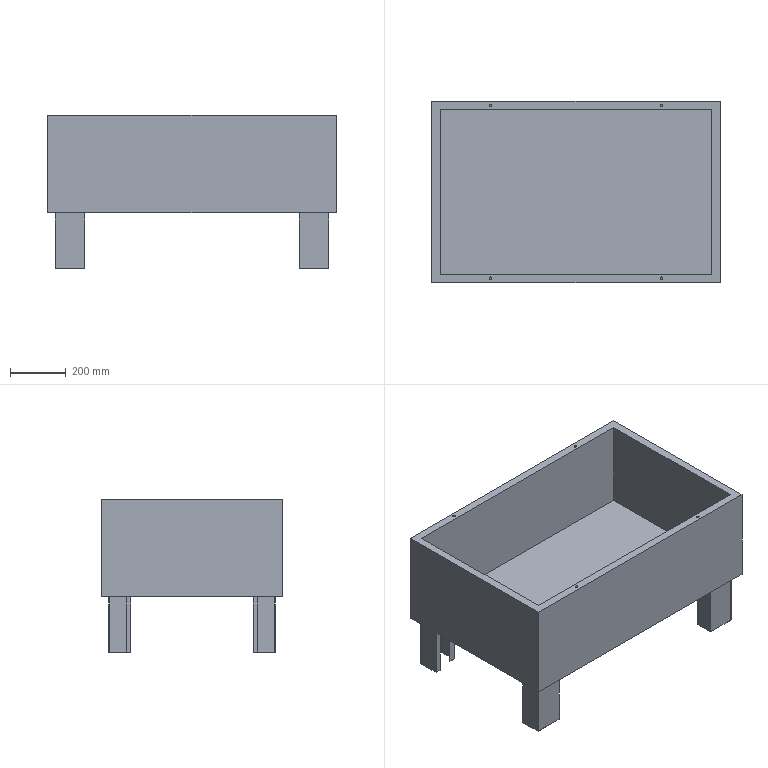Part | STEP file | 1 solid | 78 faces | box 1034 x 650 x 550 mm | volume 52186602 mm3 | plane 68 | cylinder 10 | commonest cylinder face diameters 10 x10